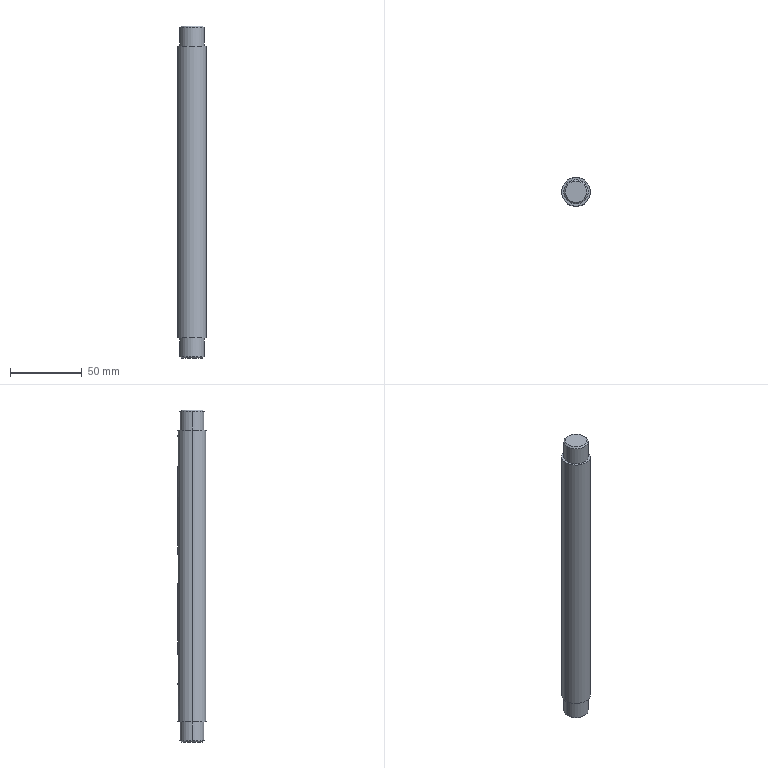Part | NX | features BREP 1 | 1 solid | 32 faces | box 20 x 20 x 231.5 mm | volume 68985 mm3 | cylinder 15 | plane 13 | cone 4 | commonest cylinder face diameters 6 x9 17 x4 20 x2
STEP:
#1=CARTESIAN_POINT('',(8.5,0.,-114.75));
#2=VERTEX_POINT('',#1);
#3=CARTESIAN_POINT('',(-8.5,0.,-114.75));
#4=VERTEX_POINT('',#3);
#5=CARTESIAN_POINT('',(0.,0.,-114.75));
#6=DIRECTION('',(0.,0.,-1.));
#7=DIRECTION('',(1.,0.,0.));
#8=AXIS2_PLACEMENT_3D('',#5,#6,#7);
#9=CIRCLE('',#8,8.5);
#10=EDGE_CURVE('',#2,#4,#9,.T.);
#11=ORIENTED_EDGE('',*,*,#10,.F.);
#12=CARTESIAN_POINT('',(8.5,0.,-101.75));
#13=VERTEX_POINT('',#12);
#14=CARTESIAN_POINT('',(8.5,0.,-101.75));
#15=DIRECTION('',(0.,0.,-1.));
#16=VECTOR('',#15,1000.);
#17=LINE('',#14,#16);
#18=EDGE_CURVE('',#13,#2,#17,.T.);
#19=ORIENTED_EDGE('',*,*,#18,.F.);
#20=CARTESIAN_POINT('',(-8.5,0.,-101.75));
#21=VERTEX_POINT('',#20);
#22=CARTESIAN_POINT('',(0.,0.,-101.75));
#23=DIRECTION('',(0.,0.,1.));
#24=DIRECTION('',(-1.,0.,0.));
#25=AXIS2_PLACEMENT_3D('',#22,#23,#24);
#26=CIRCLE('',#25,8.5);
#27=EDGE_CURVE('',#21,#13,#26,.T.);
#28=ORIENTED_EDGE('',*,*,#27,.F.);
#29=CARTESIAN_POINT('',(-8.5,0.,-101.75));
#30=DIRECTION('',(0.,0.,-1.));
#31=VECTOR('',#30,1000.);
#32=LINE('',#29,#31);
#33=EDGE_CURVE('',#21,#4,#32,.T.);
#34=ORIENTED_EDGE('',*,*,#33,.T.);
#35=EDGE_LOOP('',(#11,#19,#28,#34));
#36=FACE_BOUND('',#35,.T.);
#37=CARTESIAN_POINT('',(0.,0.,-115.75));
#38=DIRECTION('',(0.,0.,1.));
#39=DIRECTION('',(-1.,0.,0.));
#40=AXIS2_PLACEMENT_3D('',#37,#38,#39);
#41=CYLINDRICAL_SURFACE('',#40,8.5);
#42=ADVANCED_FACE('',(#36),#41,.T.);
#43=ORIENTED_EDGE('',*,*,#33,.F.);
#44=CARTESIAN_POINT('',(0.,0.,-101.75));
#45=DIRECTION('',(0.,0.,1.));
#46=DIRECTION('',(1.,0.,0.));
#47=AXIS2_PLACEMENT_3D('',#44,#45,#46);
#48=CIRCLE('',#47,8.5);
#49=EDGE_CURVE('',#13,#21,#48,.T.);
#50=ORIENTED_EDGE('',*,*,#49,.F.);
#51=ORIENTED_EDGE('',*,*,#18,.T.);
#52=CARTESIAN_POINT('',(0.,0.,-114.75));
#53=DIRECTION('',(0.,0.,-1.));
#54=DIRECTION('',(-1.,0.,0.));
#55=AXIS2_PLACEMENT_3D('',#52,#53,#54);
#56=CIRCLE('',#55,8.5);
#57=EDGE_CURVE('',#4,#2,#56,.T.);
#58=ORIENTED_EDGE('',*,*,#57,.F.);
#59=EDGE_LOOP('',(#43,#50,#51,#58));
#60=FACE_BOUND('',#59,.T.);
#61=CARTESIAN_POINT('',(0.,0.,-115.75));
#62=DIRECTION('',(0.,0.,1.));
#63=DIRECTION('',(-1.,0.,0.));
#64=AXIS2_PLACEMENT_3D('',#61,#62,#63);
#65=CYLINDRICAL_SURFACE('',#64,8.5);
#66=ADVANCED_FACE('',(#60),#65,.T.);
#67=CARTESIAN_POINT('',(-7.5,0.,-115.75));
#68=VERTEX_POINT('',#67);
#69=CARTESIAN_POINT('',(-8.5,0.,-114.75));
#70=DIRECTION('',(0.7071,0.,-0.7071));
#71=VECTOR('',#70,1000.);
#72=LINE('',#69,#71);
#73=EDGE_CURVE('',#68,#4,#72,.F.);
#74=ORIENTED_EDGE('',*,*,#73,.T.);
#75=ORIENTED_EDGE('',*,*,#57,.T.);
#76=CARTESIAN_POINT('',(7.5,0.,-115.75));
#77=VERTEX_POINT('',#76);
#78=CARTESIAN_POINT('',(8.5,0.,-114.75));
#79=DIRECTION('',(-0.7071,0.,-0.7071));
#80=VECTOR('',#79,1000.);
#81=LINE('',#78,#80);
#82=EDGE_CURVE('',#77,#2,#81,.F.);
#83=ORIENTED_EDGE('',*,*,#82,.F.);
#84=CARTESIAN_POINT('',(0.,0.,-115.75));
#85=DIRECTION('',(0.,0.,-1.));
#86=DIRECTION('',(-1.,0.,0.));
#87=AXIS2_PLACEMENT_3D('',#84,#85,#86);
#88=CIRCLE('',#87,7.5);
#89=EDGE_CURVE('',#68,#77,#88,.T.);
#90=ORIENTED_EDGE('',*,*,#89,.F.);
#91=EDGE_LOOP('',(#74,#75,#83,#90));
#92=FACE_BOUND('',#91,.T.);
#93=CARTESIAN_POINT('',(0.,0.,-115.25));
#94=DIRECTION('',(0.,0.,1.));
#95=DIRECTION('',(-1.,0.,0.));
#96=AXIS2_PLACEMENT_3D('',#93,#94,#95);
#97=CONICAL_SURFACE('',#96,8.,0.7854);
#98=ADVANCED_FACE('',(#92),#97,.T.);
#99=ORIENTED_EDGE('',*,*,#89,.T.);
#100=CARTESIAN_POINT('',(0.,0.,-115.75));
#101=DIRECTION('',(0.,0.,-1.));
#102=DIRECTION('',(1.,0.,0.));
#103=AXIS2_PLACEMENT_3D('',#100,#101,#102);
#104=CIRCLE('',#103,7.5);
#105=EDGE_CURVE('',#77,#68,#104,.T.);
#106=ORIENTED_EDGE('',*,*,#105,.T.);
#107=EDGE_LOOP('',(#99,#106));
#108=FACE_BOUND('',#107,.T.);
#109=CARTESIAN_POINT('',(0.,0.,-115.75));
#110=DIRECTION('',(0.,0.,-1.));
#111=DIRECTION('',(-1.,0.,0.));
#112=AXIS2_PLACEMENT_3D('',#109,#110,#111);
#113=PLANE('',#112);
#114=ADVANCED_FACE('',(#108),#113,.T.);
#115=ORIENTED_EDGE('',*,*,#105,.F.);
#116=ORIENTED_EDGE('',*,*,#82,.T.);
#117=ORIENTED_EDGE('',*,*,#10,.T.);
#118=ORIENTED_EDGE('',*,*,#73,.F.);
#119=EDGE_LOOP('',(#115,#116,#117,#118));
#120=FACE_BOUND('',#119,.T.);
#121=CARTESIAN_POINT('',(0.,0.,-115.25));
#122=DIRECTION('',(0.,0.,1.));
#123=DIRECTION('',(-1.,0.,0.));
#124=AXIS2_PLACEMENT_3D('',#121,#122,#123);
#125=CONICAL_SURFACE('',#124,8.,0.7854);
#126=ADVANCED_FACE('',(#120),#125,.T.);
#127=CARTESIAN_POINT('',(-10.,0.,-101.75));
#128=VERTEX_POINT('',#127);
#129=CARTESIAN_POINT('',(10.,0.,-101.75));
#130=VERTEX_POINT('',#129);
#131=CARTESIAN_POINT('',(0.,0.,-101.75));
#132=DIRECTION('',(0.,0.,-1.));
#133=DIRECTION('',(-1.,0.,0.));
#134=AXIS2_PLACEMENT_3D('',#131,#132,#133);
#135=CIRCLE('',#134,10.);
#136=EDGE_CURVE('',#128,#130,#135,.T.);
#137=ORIENTED_EDGE('',*,*,#136,.T.);
#138=CARTESIAN_POINT('',(0.,0.,-101.75));
#139=DIRECTION('',(0.,0.,-1.));
#140=DIRECTION('',(1.,0.,0.));
#141=AXIS2_PLACEMENT_3D('',#138,#139,#140);
#142=CIRCLE('',#141,10.);
#143=EDGE_CURVE('',#130,#128,#142,.T.);
#144=ORIENTED_EDGE('',*,*,#143,.T.);
#145=EDGE_LOOP('',(#137,#144));
#146=FACE_BOUND('',#145,.T.);
#147=ORIENTED_EDGE('',*,*,#27,.T.);
#148=ORIENTED_EDGE('',*,*,#49,.T.);
#149=EDGE_LOOP('',(#147,#148));
#150=FACE_BOUND('',#149,.T.);
#151=CARTESIAN_POINT('',(0.,0.,-101.75));
#152=DIRECTION('',(0.,0.,1.));
#153=DIRECTION('',(-1.,0.,0.));
#154=AXIS2_PLACEMENT_3D('',#151,#152,#153);
#155=PLANE('',#154);
#156=ADVANCED_FACE('',(#146,#150),#155,.F.);
#157=CARTESIAN_POINT('',(-10.,0.,101.75));
#158=VERTEX_POINT('',#157);
#159=CARTESIAN_POINT('',(10.,0.,101.75));
#160=VERTEX_POINT('',#159);
#161=CARTESIAN_POINT('',(0.,0.,101.75));
#162=DIRECTION('',(0.,0.,1.));
#163=DIRECTION('',(-1.,0.,0.));
#164=AXIS2_PLACEMENT_3D('',#161,#162,#163);
#165=CIRCLE('',#164,10.);
#166=EDGE_CURVE('',#158,#160,#165,.T.);
#167=ORIENTED_EDGE('',*,*,#166,.F.);
#168=CARTESIAN_POINT('',(-10.,0.,-101.75));
#169=DIRECTION('',(0.,0.,1.));
#170=VECTOR('',#169,1000.);
#171=LINE('',#168,#170);
#172=EDGE_CURVE('',#158,#128,#171,.F.);
#173=ORIENTED_EDGE('',*,*,#172,.T.);
#174=ORIENTED_EDGE('',*,*,#143,.F.);
#175=CARTESIAN_POINT('',(10.,0.,-101.75));
#176=DIRECTION('',(0.,0.,1.));
#177=VECTOR('',#176,1000.);
#178=LINE('',#175,#177);
#179=EDGE_CURVE('',#160,#130,#178,.F.);
#180=ORIENTED_EDGE('',*,*,#179,.F.);
#181=EDGE_LOOP('',(#167,#173,#174,#180));
#182=FACE_BOUND('',#181,.T.);
#183=CARTESIAN_POINT('',(0.,0.,101.75));
#184=DIRECTION('',(0.,0.,-1.));
#185=DIRECTION('',(1.,0.,0.));
#186=AXIS2_PLACEMENT_3D('',#183,#184,#185);
#187=CYLINDRICAL_SURFACE('',#186,10.);
#188=ADVANCED_FACE('',(#182),#187,.T.);
#189=ORIENTED_EDGE('',*,*,#179,.T.);
#190=ORIENTED_EDGE('',*,*,#136,.F.);
#191=ORIENTED_EDGE('',*,*,#172,.F.);
#192=CARTESIAN_POINT('',(0.,0.,101.75));
#193=DIRECTION('',(0.,0.,1.));
#194=DIRECTION('',(1.,0.,0.));
#195=AXIS2_PLACEMENT_3D('',#192,#193,#194);
#196=CIRCLE('',#195,10.);
#197=EDGE_CURVE('',#160,#158,#196,.T.);
#198=ORIENTED_EDGE('',*,*,#197,.F.);
#199=EDGE_LOOP('',(#189,#190,#191,#198));
#200=FACE_BOUND('',#199,.T.);
#201=CARTESIAN_POINT('',(-3.,9.539,94.75));
#202=VERTEX_POINT('',#201);
#203=CARTESIAN_POINT('',(0.,10.,97.75));
#204=VERTEX_POINT('',#203);
#205=CARTESIAN_POINT('',(-3.,9.539,94.75));
#206=CARTESIAN_POINT('',(-3.,9.539,95.547));
#207=CARTESIAN_POINT('',(-2.345,9.775,97.093));
#208=CARTESIAN_POINT('',(-0.7973,10.,97.75));
#209=CARTESIAN_POINT('',(0.,10.,97.75));
#210=B_SPLINE_CURVE_WITH_KNOTS('',3,(#205,#206,#207,#208,#209),.UNSPECIFIED.,.F.,.F.,(4,1,4),(0.,0.002357,0.004714),.UNSPECIFIED.);
#211=EDGE_CURVE('',#202,#204,#210,.T.);
#212=ORIENTED_EDGE('',*,*,#211,.F.);
#213=CARTESIAN_POINT('',(-3.,9.539,78.75));
#214=VERTEX_POINT('',#213);
#215=CARTESIAN_POINT('',(-3.,9.539,94.75));
#216=DIRECTION('',(0.,0.,-1.));
#217=VECTOR('',#216,1000.);
#218=LINE('',#215,#217);
#219=EDGE_CURVE('',#202,#214,#218,.T.);
#220=ORIENTED_EDGE('',*,*,#219,.T.);
#221=CARTESIAN_POINT('',(3.,9.539,78.75));
#222=VERTEX_POINT('',#221);
#223=CARTESIAN_POINT('',(3.,9.539,78.75));
#224=CARTESIAN_POINT('',(3.,9.539,77.952));
#225=CARTESIAN_POINT('',(2.35,9.775,76.406));
#226=CARTESIAN_POINT('',(0.004774,10.112,75.422));
#227=CARTESIAN_POINT('',(-2.351,9.775,76.405));
#228=CARTESIAN_POINT('',(-3.,9.539,77.952));
#229=CARTESIAN_POINT('',(-3.,9.539,78.75));
#230=B_SPLINE_CURVE_WITH_KNOTS('',3,(#223,#224,#225,#226,#227,#228,#229),.UNSPECIFIED.,.F.,.F.,(4,1,1,1,4),(0.,0.002358,0.004715,0.007073,0.009431),.UNSPECIFIED.);
#231=EDGE_CURVE('',#222,#214,#230,.T.);
#232=ORIENTED_EDGE('',*,*,#231,.F.);
#233=CARTESIAN_POINT('',(3.,9.539,94.75));
#234=VERTEX_POINT('',#233);
#235=CARTESIAN_POINT('',(3.,9.539,78.75));
#236=DIRECTION('',(0.,0.,1.));
#237=VECTOR('',#236,1000.);
#238=LINE('',#235,#237);
#239=EDGE_CURVE('',#222,#234,#238,.T.);
#240=ORIENTED_EDGE('',*,*,#239,.T.);
#241=CARTESIAN_POINT('',(0.,10.,97.75));
#242=CARTESIAN_POINT('',(0.7973,10.,97.75));
#243=CARTESIAN_POINT('',(2.343,9.775,97.095));
#244=CARTESIAN_POINT('',(3.,9.539,95.547));
#245=CARTESIAN_POINT('',(3.,9.539,94.75));
#246=B_SPLINE_CURVE_WITH_KNOTS('',3,(#241,#242,#243,#244,#245),.UNSPECIFIED.,.F.,.F.,(4,1,4),(0.,0.002357,0.004714),.UNSPECIFIED.);
#247=EDGE_CURVE('',#204,#234,#246,.T.);
#248=ORIENTED_EDGE('',*,*,#247,.F.);
#249=EDGE_LOOP('',(#212,#220,#232,#240,#248));
#250=FACE_BOUND('',#249,.T.);
#251=CARTESIAN_POINT('',(-3.,9.539,-56.75));
#252=VERTEX_POINT('',#251);
#253=CARTESIAN_POINT('',(0.,10.,-53.75));
#254=VERTEX_POINT('',#253);
#255=CARTESIAN_POINT('',(-3.,9.539,-56.75));
#256=CARTESIAN_POINT('',(-3.,9.539,-55.953));
#257=CARTESIAN_POINT('',(-2.345,9.775,-54.407));
#258=CARTESIAN_POINT('',(-0.7973,10.,-53.75));
#259=CARTESIAN_POINT('',(0.,10.,-53.75));
#260=B_SPLINE_CURVE_WITH_KNOTS('',3,(#255,#256,#257,#258,#259),.UNSPECIFIED.,.F.,.F.,(4,1,4),(0.,0.002357,0.004714),.UNSPECIFIED.);
#261=EDGE_CURVE('',#252,#254,#260,.T.);
#262=ORIENTED_EDGE('',*,*,#261,.F.);
#263=CARTESIAN_POINT('',(-3.,9.539,-72.75));
#264=VERTEX_POINT('',#263);
#265=CARTESIAN_POINT('',(-3.,9.539,-56.75));
#266=DIRECTION('',(0.,0.,-1.));
#267=VECTOR('',#266,1000.);
#268=LINE('',#265,#267);
#269=EDGE_CURVE('',#252,#264,#268,.T.);
#270=ORIENTED_EDGE('',*,*,#269,.T.);
#271=CARTESIAN_POINT('',(3.,9.539,-72.75));
#272=VERTEX_POINT('',#271);
#273=CARTESIAN_POINT('',(3.,9.539,-72.75));
#274=CARTESIAN_POINT('',(3.,9.539,-73.548));
#275=CARTESIAN_POINT('',(2.35,9.775,-75.094));
#276=CARTESIAN_POINT('',(0.004774,10.112,-76.078));
#277=CARTESIAN_POINT('',(-2.351,9.775,-75.095));
#278=CARTESIAN_POINT('',(-3.,9.539,-73.548));
#279=CARTESIAN_POINT('',(-3.,9.539,-72.75));
#280=B_SPLINE_CURVE_WITH_KNOTS('',3,(#273,#274,#275,#276,#277,#278,#279),.UNSPECIFIED.,.F.,.F.,(4,1,1,1,4),(0.,0.002358,0.004715,0.007073,0.009431),.UNSPECIFIED.);
#281=EDGE_CURVE('',#272,#264,#280,.T.);
#282=ORIENTED_EDGE('',*,*,#281,.F.);
#283=CARTESIAN_POINT('',(3.,9.539,-56.75));
#284=VERTEX_POINT('',#283);
#285=CARTESIAN_POINT('',(3.,9.539,-72.75));
#286=DIRECTION('',(0.,0.,1.));
#287=VECTOR('',#286,1000.);
#288=LINE('',#285,#287);
#289=EDGE_CURVE('',#272,#284,#288,.T.);
#290=ORIENTED_EDGE('',*,*,#289,.T.);
#291=CARTESIAN_POINT('',(0.,10.,-53.75));
#292=CARTESIAN_POINT('',(0.7973,10.,-53.75));
#293=CARTESIAN_POINT('',(2.343,9.775,-54.405));
#294=CARTESIAN_POINT('',(3.,9.539,-55.953));
#295=CARTESIAN_POINT('',(3.,9.539,-56.75));
#296=B_SPLINE_CURVE_WITH_KNOTS('',3,(#291,#292,#293,#294,#295),.UNSPECIFIED.,.F.,.F.,(4,1,4),(0.,0.002357,0.004714),.UNSPECIFIED.);
#297=EDGE_CURVE('',#254,#284,#296,.T.);
#298=ORIENTED_EDGE('',*,*,#297,.F.);
#299=EDGE_LOOP('',(#262,#270,#282,#290,#298));
#300=FACE_BOUND('',#299,.T.);
#301=CARTESIAN_POINT('',(-3.,9.539,13.));
#302=VERTEX_POINT('',#301);
#303=CARTESIAN_POINT('',(0.,10.,16.));
#304=VERTEX_POINT('',#303);
#305=CARTESIAN_POINT('',(-3.,9.539,13.));
#306=CARTESIAN_POINT('',(-3.,9.539,13.797));
#307=CARTESIAN_POINT('',(-2.345,9.775,15.343));
#308=CARTESIAN_POINT('',(-0.7973,10.,16.));
#309=CARTESIAN_POINT('',(0.,10.,16.));
#310=B_SPLINE_CURVE_WITH_KNOTS('',3,(#305,#306,#307,#308,#309),.UNSPECIFIED.,.F.,.F.,(4,1,4),(0.,0.002357,0.004714),.UNSPECIFIED.);
#311=EDGE_CURVE('',#302,#304,#310,.T.);
#312=ORIENTED_EDGE('',*,*,#311,.F.);
#313=CARTESIAN_POINT('',(-3.,9.539,-3.));
#314=VERTEX_POINT('',#313);
#315=CARTESIAN_POINT('',(-3.,9.539,13.));
#316=DIRECTION('',(0.,0.,-1.));
#317=VECTOR('',#316,1000.);
#318=LINE('',#315,#317);
#319=EDGE_CURVE('',#302,#314,#318,.T.);
#320=ORIENTED_EDGE('',*,*,#319,.T.);
#321=CARTESIAN_POINT('',(3.,9.539,-3.));
#322=VERTEX_POINT('',#321);
#323=CARTESIAN_POINT('',(3.,9.539,-3.));
#324=CARTESIAN_POINT('',(3.,9.539,-3.798));
#325=CARTESIAN_POINT('',(2.35,9.775,-5.344));
#326=CARTESIAN_POINT('',(0.004774,10.112,-6.328));
#327=CARTESIAN_POINT('',(-2.351,9.775,-5.345));
#328=CARTESIAN_POINT('',(-3.,9.539,-3.798));
#329=CARTESIAN_POINT('',(-3.,9.539,-3.));
#330=B_SPLINE_CURVE_WITH_KNOTS('',3,(#323,#324,#325,#326,#327,#328,#329),.UNSPECIFIED.,.F.,.F.,(4,1,1,1,4),(0.,0.002358,0.004715,0.007073,0.009431),.UNSPECIFIED.);
#331=EDGE_CURVE('',#322,#314,#330,.T.);
#332=ORIENTED_EDGE('',*,*,#331,.F.);
#333=CARTESIAN_POINT('',(3.,9.539,13.));
#334=VERTEX_POINT('',#333);
#335=CARTESIAN_POINT('',(3.,9.539,-3.));
#336=DIRECTION('',(0.,0.,1.));
#337=VECTOR('',#336,1000.);
#338=LINE('',#335,#337);
#339=EDGE_CURVE('',#322,#334,#338,.T.);
#340=ORIENTED_EDGE('',*,*,#339,.T.);
#341=CARTESIAN_POINT('',(0.,10.,16.));
#342=CARTESIAN_POINT('',(0.7973,10.,16.));
#343=CARTESIAN_POINT('',(2.343,9.775,15.345));
#344=CARTESIAN_POINT('',(3.,9.539,13.797));
#345=CARTESIAN_POINT('',(3.,9.539,13.));
#346=B_SPLINE_CURVE_WITH_KNOTS('',3,(#341,#342,#343,#344,#345),.UNSPECIFIED.,.F.,.F.,(4,1,4),(0.,0.002357,0.004714),.UNSPECIFIED.);
#347=EDGE_CURVE('',#304,#334,#346,.T.);
#348=ORIENTED_EDGE('',*,*,#347,.F.);
#349=EDGE_LOOP('',(#312,#320,#332,#340,#348));
#350=FACE_BOUND('',#349,.T.);
#351=CARTESIAN_POINT('',(0.,0.,101.75));
#352=DIRECTION('',(0.,0.,-1.));
#353=DIRECTION('',(1.,0.,0.));
#354=AXIS2_PLACEMENT_3D('',#351,#352,#353);
#355=CYLINDRICAL_SURFACE('',#354,10.);
#356=ADVANCED_FACE('',(#200,#250,#300,#350),#355,.T.);
#357=ORIENTED_EDGE('',*,*,#197,.T.);
#358=ORIENTED_EDGE('',*,*,#166,.T.);
#359=EDGE_LOOP('',(#357,#358));
#360=FACE_BOUND('',#359,.T.);
#361=CARTESIAN_POINT('',(-8.5,0.,101.75));
#362=VERTEX_POINT('',#361);
#363=CARTESIAN_POINT('',(8.5,0.,101.75));
#364=VERTEX_POINT('',#363);
#365=CARTESIAN_POINT('',(0.,0.,101.75));
#366=DIRECTION('',(0.,0.,-1.));
#367=DIRECTION('',(-1.,0.,0.));
#368=AXIS2_PLACEMENT_3D('',#365,#366,#367);
#369=CIRCLE('',#368,8.5);
#370=EDGE_CURVE('',#362,#364,#369,.T.);
#371=ORIENTED_EDGE('',*,*,#370,.T.);
#372=CARTESIAN_POINT('',(0.,0.,101.75));
#373=DIRECTION('',(0.,0.,-1.));
#374=DIRECTION('',(1.,0.,0.));
#375=AXIS2_PLACEMENT_3D('',#372,#373,#374);
#376=CIRCLE('',#375,8.5);
#377=EDGE_CURVE('',#364,#362,#376,.T.);
#378=ORIENTED_EDGE('',*,*,#377,.T.);
#379=EDGE_LOOP('',(#371,#378));
#380=FACE_BOUND('',#379,.T.);
#381=CARTESIAN_POINT('',(0.,0.,101.75));
#382=DIRECTION('',(0.,0.,1.));
#383=DIRECTION('',(-1.,0.,0.));
#384=AXIS2_PLACEMENT_3D('',#381,#382,#383);
#385=PLANE('',#384);
#386=ADVANCED_FACE('',(#360,#380),#385,.T.);
#387=CARTESIAN_POINT('',(-8.5,0.,114.75));
#388=VERTEX_POINT('',#387);
#389=CARTESIAN_POINT('',(8.5,0.,114.75));
#390=VERTEX_POINT('',#389);
#391=CARTESIAN_POINT('',(0.,0.,114.75));
#392=DIRECTION('',(0.,0.,1.));
#393=DIRECTION('',(-1.,0.,0.));
#394=AXIS2_PLACEMENT_3D('',#391,#392,#393);
#395=CIRCLE('',#394,8.5);
#396=EDGE_CURVE('',#388,#390,#395,.T.);
#397=ORIENTED_EDGE('',*,*,#396,.F.);
#398=CARTESIAN_POINT('',(-8.5,0.,101.75));
#399=DIRECTION('',(0.,0.,1.));
#400=VECTOR('',#399,1000.);
#401=LINE('',#398,#400);
#402=EDGE_CURVE('',#388,#362,#401,.F.);
#403=ORIENTED_EDGE('',*,*,#402,.T.);
#404=ORIENTED_EDGE('',*,*,#377,.F.);
#405=CARTESIAN_POINT('',(8.5,0.,101.75));
#406=DIRECTION('',(0.,0.,1.));
#407=VECTOR('',#406,1000.);
#408=LINE('',#405,#407);
#409=EDGE_CURVE('',#390,#364,#408,.F.);
#410=ORIENTED_EDGE('',*,*,#409,.F.);
#411=EDGE_LOOP('',(#397,#403,#404,#410));
#412=FACE_BOUND('',#411,.T.);
#413=CARTESIAN_POINT('',(0.,0.,115.75));
#414=DIRECTION('',(0.,0.,-1.));
#415=DIRECTION('',(1.,0.,0.));
#416=AXIS2_PLACEMENT_3D('',#413,#414,#415);
#417=CYLINDRICAL_SURFACE('',#416,8.5);
#418=ADVANCED_FACE('',(#412),#417,.T.);
#419=ORIENTED_EDGE('',*,*,#409,.T.);
#420=ORIENTED_EDGE('',*,*,#370,.F.);
#421=ORIENTED_EDGE('',*,*,#402,.F.);
#422=CARTESIAN_POINT('',(0.,0.,114.75));
#423=DIRECTION('',(0.,0.,1.));
#424=DIRECTION('',(1.,0.,0.));
#425=AXIS2_PLACEMENT_3D('',#422,#423,#424);
#426=CIRCLE('',#425,8.5);
#427=EDGE_CURVE('',#390,#388,#426,.T.);
#428=ORIENTED_EDGE('',*,*,#427,.F.);
#429=EDGE_LOOP('',(#419,#420,#421,#428));
#430=FACE_BOUND('',#429,.T.);
#431=CARTESIAN_POINT('',(0.,0.,115.75));
#432=DIRECTION('',(0.,0.,-1.));
#433=DIRECTION('',(1.,0.,0.));
#434=AXIS2_PLACEMENT_3D('',#431,#432,#433);
#435=CYLINDRICAL_SURFACE('',#434,8.5);
#436=ADVANCED_FACE('',(#430),#435,.T.);
#437=CARTESIAN_POINT('',(7.5,0.,115.75));
#438=VERTEX_POINT('',#437);
#439=CARTESIAN_POINT('',(8.5,0.,114.75));
#440=DIRECTION('',(-0.7071,0.,0.7071));
#441=VECTOR('',#440,1000.);
#442=LINE('',#439,#441);
#443=EDGE_CURVE('',#390,#438,#442,.T.);
#444=ORIENTED_EDGE('',*,*,#443,.F.);
#445=ORIENTED_EDGE('',*,*,#427,.T.);
#446=CARTESIAN_POINT('',(-7.5,0.,115.75));
#447=VERTEX_POINT('',#446);
#448=CARTESIAN_POINT('',(-8.5,0.,114.75));
#449=DIRECTION('',(0.7071,0.,0.7071));
#450=VECTOR('',#449,1000.);
#451=LINE('',#448,#450);
#452=EDGE_CURVE('',#388,#447,#451,.T.);
#453=ORIENTED_EDGE('',*,*,#452,.T.);
#454=CARTESIAN_POINT('',(0.,0.,115.75));
#455=DIRECTION('',(0.,0.,1.));
#456=DIRECTION('',(1.,0.,0.));
#457=AXIS2_PLACEMENT_3D('',#454,#455,#456);
#458=CIRCLE('',#457,7.5);
#459=EDGE_CURVE('',#438,#447,#458,.T.);
#460=ORIENTED_EDGE('',*,*,#459,.F.);
#461=EDGE_LOOP('',(#444,#445,#453,#460));
#462=FACE_BOUND('',#461,.T.);
#463=CARTESIAN_POINT('',(0.,0.,115.25));
#464=DIRECTION('',(0.,0.,-1.));
#465=DIRECTION('',(1.,0.,0.));
#466=AXIS2_PLACEMENT_3D('',#463,#464,#465);
#467=CONICAL_SURFACE('',#466,8.,0.7854);
#468=ADVANCED_FACE('',(#462),#467,.T.);
#469=ORIENTED_EDGE('',*,*,#459,.T.);
#470=CARTESIAN_POINT('',(0.,0.,115.75));
#471=DIRECTION('',(0.,0.,1.));
#472=DIRECTION('',(-1.,0.,0.));
#473=AXIS2_PLACEMENT_3D('',#470,#471,#472);
#474=CIRCLE('',#473,7.5);
#475=EDGE_CURVE('',#447,#438,#474,.T.);
#476=ORIENTED_EDGE('',*,*,#475,.T.);
#477=EDGE_LOOP('',(#469,#476));
#478=FACE_BOUND('',#477,.T.);
#479=CARTESIAN_POINT('',(0.,0.,115.75));
#480=DIRECTION('',(0.,0.,1.));
#481=DIRECTION('',(-1.,0.,0.));
#482=AXIS2_PLACEMENT_3D('',#479,#480,#481);
#483=PLANE('',#482);
#484=ADVANCED_FACE('',(#478),#483,.T.);
#485=ORIENTED_EDGE('',*,*,#475,.F.);
#486=ORIENTED_EDGE('',*,*,#452,.F.);
#487=ORIENTED_EDGE('',*,*,#396,.T.);
#488=ORIENTED_EDGE('',*,*,#443,.T.);
#489=EDGE_LOOP('',(#485,#486,#487,#488));
#490=FACE_BOUND('',#489,.T.);
#491=CARTESIAN_POINT('',(0.,0.,115.25));
#492=DIRECTION('',(0.,0.,-1.));
#493=DIRECTION('',(1.,0.,0.));
#494=AXIS2_PLACEMENT_3D('',#491,#492,#493);
#495=CONICAL_SURFACE('',#494,8.,0.7854);
#496=ADVANCED_FACE('',(#490),#495,.T.);
#497=CARTESIAN_POINT('',(0.,6.5,97.75));
#498=VERTEX_POINT('',#497);
#499=CARTESIAN_POINT('',(0.,10.,97.75));
#500=DIRECTION('',(0.,-1.,0.));
#501=VECTOR('',#500,1000.);
#502=LINE('',#499,#501);
#503=EDGE_CURVE('',#204,#498,#502,.T.);
#504=ORIENTED_EDGE('',*,*,#503,.F.);
#505=ORIENTED_EDGE('',*,*,#247,.T.);
#506=CARTESIAN_POINT('',(3.,6.5,94.75));
#507=VERTEX_POINT('',#506);
#508=CARTESIAN_POINT('',(3.,9.539,94.75));
#509=DIRECTION('',(0.,-1.,0.));
#510=VECTOR('',#509,1000.);
#511=LINE('',#508,#510);
#512=EDGE_CURVE('',#234,#507,#511,.T.);
#513=ORIENTED_EDGE('',*,*,#512,.T.);
#514=CARTESIAN_POINT('',(0.,6.5,94.75));
#515=DIRECTION('',(0.,1.,0.));
#516=DIRECTION('',(0.,0.,1.));
#517=AXIS2_PLACEMENT_3D('',#514,#515,#516);
#518=CIRCLE('',#517,3.);
#519=EDGE_CURVE('',#498,#507,#518,.T.);
#520=ORIENTED_EDGE('',*,*,#519,.F.);
#521=EDGE_LOOP('',(#504,#505,#513,#520));
#522=FACE_BOUND('',#521,.T.);
#523=CARTESIAN_POINT('',(0.,6.5,94.75));
#524=DIRECTION('',(0.,1.,0.));
#525=DIRECTION('',(0.,0.,-1.));
#526=AXIS2_PLACEMENT_3D('',#523,#524,#525);
#527=CYLINDRICAL_SURFACE('',#526,3.);
#528=ADVANCED_FACE('',(#522),#527,.F.);
#529=CARTESIAN_POINT('',(0.,6.5,75.75));
#530=VERTEX_POINT('',#529);
#531=CARTESIAN_POINT('',(-3.,6.5,78.75));
#532=VERTEX_POINT('',#531);
#533=CARTESIAN_POINT('',(0.,6.5,78.75));
#534=DIRECTION('',(0.,1.,0.));
#535=DIRECTION('',(0.,0.,-1.));
#536=AXIS2_PLACEMENT_3D('',#533,#534,#535);
#537=CIRCLE('',#536,3.);
#538=EDGE_CURVE('',#530,#532,#537,.T.);
#539=ORIENTED_EDGE('',*,*,#538,.T.);
#540=CARTESIAN_POINT('',(-3.,6.5,94.75));
#541=VERTEX_POINT('',#540);
#542=CARTESIAN_POINT('',(-3.,6.5,94.75));
#543=DIRECTION('',(0.,0.,-1.));
#544=VECTOR('',#543,1000.);
#545=LINE('',#542,#544);
#546=EDGE_CURVE('',#541,#532,#545,.T.);
#547=ORIENTED_EDGE('',*,*,#546,.F.);
#548=CARTESIAN_POINT('',(0.,6.5,94.75));
#549=DIRECTION('',(0.,1.,0.));
#550=DIRECTION('',(-1.,0.,0.));
#551=AXIS2_PLACEMENT_3D('',#548,#549,#550);
#552=CIRCLE('',#551,3.);
#553=EDGE_CURVE('',#541,#498,#552,.T.);
#554=ORIENTED_EDGE('',*,*,#553,.T.);
#555=ORIENTED_EDGE('',*,*,#519,.T.);
#556=CARTESIAN_POINT('',(3.,6.5,78.75));
#557=VERTEX_POINT('',#556);
#558=CARTESIAN_POINT('',(3.,6.5,78.75));
#559=DIRECTION('',(0.,0.,1.));
#560=VECTOR('',#559,1000.);
#561=LINE('',#558,#560);
#562=EDGE_CURVE('',#557,#507,#561,.T.);
#563=ORIENTED_EDGE('',*,*,#562,.F.);
#564=CARTESIAN_POINT('',(0.,6.5,78.75));
#565=DIRECTION('',(0.,1.,0.));
#566=DIRECTION('',(1.,0.,0.));
#567=AXIS2_PLACEMENT_3D('',#564,#565,#566);
#568=CIRCLE('',#567,3.);
#569=EDGE_CURVE('',#557,#530,#568,.T.);
#570=ORIENTED_EDGE('',*,*,#569,.T.);
#571=EDGE_LOOP('',(#539,#547,#554,#555,#563,#570));
#572=FACE_BOUND('',#571,.T.);
#573=CARTESIAN_POINT('',(0.,6.5,78.75));
#574=DIRECTION('',(0.,1.,0.));
#575=DIRECTION('',(0.,0.,-1.));
#576=AXIS2_PLACEMENT_3D('',#573,#574,#575);
#577=PLANE('',#576);
#578=ADVANCED_FACE('',(#572),#577,.T.);
#579=ORIENTED_EDGE('',*,*,#538,.F.);
#580=ORIENTED_EDGE('',*,*,#569,.F.);
#581=CARTESIAN_POINT('',(3.,6.5,78.75));
#582=DIRECTION('',(0.,1.,0.));
#583=VECTOR('',#582,1000.);
#584=LINE('',#581,#583);
#585=EDGE_CURVE('',#557,#222,#584,.T.);
#586=ORIENTED_EDGE('',*,*,#585,.T.);
#587=ORIENTED_EDGE('',*,*,#231,.T.);
#588=CARTESIAN_POINT('',(-3.,9.539,78.75));
#589=DIRECTION('',(0.,-1.,0.));
#590=VECTOR('',#589,1000.);
#591=LINE('',#588,#590);
#592=EDGE_CURVE('',#214,#532,#591,.T.);
#593=ORIENTED_EDGE('',*,*,#592,.T.);
#594=EDGE_LOOP('',(#579,#580,#586,#587,#593));
#595=FACE_BOUND('',#594,.T.);
#596=CARTESIAN_POINT('',(0.,6.5,78.75));
#597=DIRECTION('',(0.,1.,0.));
#598=DIRECTION('',(0.,0.,-1.));
#599=AXIS2_PLACEMENT_3D('',#596,#597,#598);
#600=CYLINDRICAL_SURFACE('',#599,3.);
#601=ADVANCED_FACE('',(#595),#600,.F.);
#602=ORIENTED_EDGE('',*,*,#546,.T.);
#603=ORIENTED_EDGE('',*,*,#592,.F.);
#604=ORIENTED_EDGE('',*,*,#219,.F.);
#605=CARTESIAN_POINT('',(-3.,6.5,94.75));
#606=DIRECTION('',(0.,1.,0.));
#607=VECTOR('',#606,1000.);
#608=LINE('',#605,#607);
#609=EDGE_CURVE('',#541,#202,#608,.T.);
#610=ORIENTED_EDGE('',*,*,#609,.F.);
#611=EDGE_LOOP('',(#602,#603,#604,#610));
#612=FACE_BOUND('',#611,.T.);
#613=CARTESIAN_POINT('',(-3.,6.5,78.75));
#614=DIRECTION('',(-1.,0.,0.));
#615=DIRECTION('',(0.,0.,-1.));
#616=AXIS2_PLACEMENT_3D('',#613,#614,#615);
#617=PLANE('',#616);
#618=ADVANCED_FACE('',(#612),#617,.F.);
#619=ORIENTED_EDGE('',*,*,#553,.F.);
#620=ORIENTED_EDGE('',*,*,#609,.T.);
#621=ORIENTED_EDGE('',*,*,#211,.T.);
#622=ORIENTED_EDGE('',*,*,#503,.T.);
#623=EDGE_LOOP('',(#619,#620,#621,#622));
#624=FACE_BOUND('',#623,.T.);
#625=CARTESIAN_POINT('',(0.,6.5,94.75));
#626=DIRECTION('',(0.,1.,0.));
#627=DIRECTION('',(0.,0.,-1.));
#628=AXIS2_PLACEMENT_3D('',#625,#626,#627);
#629=CYLINDRICAL_SURFACE('',#628,3.);
#630=ADVANCED_FACE('',(#624),#629,.F.);
#631=ORIENTED_EDGE('',*,*,#562,.T.);
#632=ORIENTED_EDGE('',*,*,#512,.F.);
#633=ORIENTED_EDGE('',*,*,#239,.F.);
#634=ORIENTED_EDGE('',*,*,#585,.F.);
#635=EDGE_LOOP('',(#631,#632,#633,#634));
#636=FACE_BOUND('',#635,.T.);
#637=CARTESIAN_POINT('',(3.,6.5,78.75));
#638=DIRECTION('',(1.,0.,0.));
#639=DIRECTION('',(0.,0.,1.));
#640=AXIS2_PLACEMENT_3D('',#637,#638,#639);
#641=PLANE('',#640);
#642=ADVANCED_FACE('',(#636),#641,.F.);
#643=CARTESIAN_POINT('',(0.,6.5,-53.75));
#644=VERTEX_POINT('',#643);
#645=CARTESIAN_POINT('',(0.,10.,-53.75));
#646=DIRECTION('',(0.,-1.,0.));
#647=VECTOR('',#646,1000.);
#648=LINE('',#645,#647);
#649=EDGE_CURVE('',#254,#644,#648,.T.);
#650=ORIENTED_EDGE('',*,*,#649,.F.);
#651=ORIENTED_EDGE('',*,*,#297,.T.);
#652=CARTESIAN_POINT('',(3.,6.5,-56.75));
#653=VERTEX_POINT('',#652);
#654=CARTESIAN_POINT('',(3.,9.539,-56.75));
#655=DIRECTION('',(0.,-1.,0.));
#656=VECTOR('',#655,1000.);
#657=LINE('',#654,#656);
#658=EDGE_CURVE('',#284,#653,#657,.T.);
#659=ORIENTED_EDGE('',*,*,#658,.T.);
#660=CARTESIAN_POINT('',(0.,6.5,-56.75));
#661=DIRECTION('',(0.,1.,0.));
#662=DIRECTION('',(0.,0.,1.));
#663=AXIS2_PLACEMENT_3D('',#660,#661,#662);
#664=CIRCLE('',#663,3.);
#665=EDGE_CURVE('',#644,#653,#664,.T.);
#666=ORIENTED_EDGE('',*,*,#665,.F.);
#667=EDGE_LOOP('',(#650,#651,#659,#666));
#668=FACE_BOUND('',#667,.T.);
#669=CARTESIAN_POINT('',(0.,6.5,-56.75));
#670=DIRECTION('',(0.,1.,0.));
#671=DIRECTION('',(0.,0.,-1.));
#672=AXIS2_PLACEMENT_3D('',#669,#670,#671);
#673=CYLINDRICAL_SURFACE('',#672,3.);
#674=ADVANCED_FACE('',(#668),#673,.F.);
#675=CARTESIAN_POINT('',(0.,6.5,-75.75));
#676=VERTEX_POINT('',#675);
#677=CARTESIAN_POINT('',(-3.,6.5,-72.75));
#678=VERTEX_POINT('',#677);
#679=CARTESIAN_POINT('',(0.,6.5,-72.75));
#680=DIRECTION('',(0.,1.,0.));
#681=DIRECTION('',(0.,0.,-1.));
#682=AXIS2_PLACEMENT_3D('',#679,#680,#681);
#683=CIRCLE('',#682,3.);
#684=EDGE_CURVE('',#676,#678,#683,.T.);
#685=ORIENTED_EDGE('',*,*,#684,.T.);
#686=CARTESIAN_POINT('',(-3.,6.5,-56.75));
#687=VERTEX_POINT('',#686);
#688=CARTESIAN_POINT('',(-3.,6.5,-56.75));
#689=DIRECTION('',(0.,0.,-1.));
#690=VECTOR('',#689,1000.);
#691=LINE('',#688,#690);
#692=EDGE_CURVE('',#687,#678,#691,.T.);
#693=ORIENTED_EDGE('',*,*,#692,.F.);
#694=CARTESIAN_POINT('',(0.,6.5,-56.75));
#695=DIRECTION('',(0.,1.,0.));
#696=DIRECTION('',(-1.,0.,0.));
#697=AXIS2_PLACEMENT_3D('',#694,#695,#696);
#698=CIRCLE('',#697,3.);
#699=EDGE_CURVE('',#687,#644,#698,.T.);
#700=ORIENTED_EDGE('',*,*,#699,.T.);
#701=ORIENTED_EDGE('',*,*,#665,.T.);
#702=CARTESIAN_POINT('',(3.,6.5,-72.75));
#703=VERTEX_POINT('',#702);
#704=CARTESIAN_POINT('',(3.,6.5,-72.75));
#705=DIRECTION('',(0.,0.,1.));
#706=VECTOR('',#705,1000.);
#707=LINE('',#704,#706);
#708=EDGE_CURVE('',#703,#653,#707,.T.);
#709=ORIENTED_EDGE('',*,*,#708,.F.);
#710=CARTESIAN_POINT('',(0.,6.5,-72.75));
#711=DIRECTION('',(0.,1.,0.));
#712=DIRECTION('',(1.,0.,0.));
#713=AXIS2_PLACEMENT_3D('',#710,#711,#712);
#714=CIRCLE('',#713,3.);
#715=EDGE_CURVE('',#703,#676,#714,.T.);
#716=ORIENTED_EDGE('',*,*,#715,.T.);
#717=EDGE_LOOP('',(#685,#693,#700,#701,#709,#716));
#718=FACE_BOUND('',#717,.T.);
#719=CARTESIAN_POINT('',(0.,6.5,-72.75));
#720=DIRECTION('',(0.,1.,0.));
#721=DIRECTION('',(0.,0.,-1.));
#722=AXIS2_PLACEMENT_3D('',#719,#720,#721);
#723=PLANE('',#722);
#724=ADVANCED_FACE('',(#718),#723,.T.);
#725=ORIENTED_EDGE('',*,*,#684,.F.);
#726=ORIENTED_EDGE('',*,*,#715,.F.);
#727=CARTESIAN_POINT('',(3.,6.5,-72.75));
#728=DIRECTION('',(0.,1.,0.));
#729=VECTOR('',#728,1000.);
#730=LINE('',#727,#729);
#731=EDGE_CURVE('',#703,#272,#730,.T.);
#732=ORIENTED_EDGE('',*,*,#731,.T.);
#733=ORIENTED_EDGE('',*,*,#281,.T.);
#734=CARTESIAN_POINT('',(-3.,9.539,-72.75));
#735=DIRECTION('',(0.,-1.,0.));
#736=VECTOR('',#735,1000.);
#737=LINE('',#734,#736);
#738=EDGE_CURVE('',#264,#678,#737,.T.);
#739=ORIENTED_EDGE('',*,*,#738,.T.);
#740=EDGE_LOOP('',(#725,#726,#732,#733,#739));
#741=FACE_BOUND('',#740,.T.);
#742=CARTESIAN_POINT('',(0.,6.5,-72.75));
#743=DIRECTION('',(0.,1.,0.));
#744=DIRECTION('',(0.,0.,-1.));
#745=AXIS2_PLACEMENT_3D('',#742,#743,#744);
#746=CYLINDRICAL_SURFACE('',#745,3.);
#747=ADVANCED_FACE('',(#741),#746,.F.);
#748=ORIENTED_EDGE('',*,*,#692,.T.);
#749=ORIENTED_EDGE('',*,*,#738,.F.);
#750=ORIENTED_EDGE('',*,*,#269,.F.);
#751=CARTESIAN_POINT('',(-3.,6.5,-56.75));
#752=DIRECTION('',(0.,1.,0.));
#753=VECTOR('',#752,1000.);
#754=LINE('',#751,#753);
#755=EDGE_CURVE('',#687,#252,#754,.T.);
#756=ORIENTED_EDGE('',*,*,#755,.F.);
#757=EDGE_LOOP('',(#748,#749,#750,#756));
#758=FACE_BOUND('',#757,.T.);
#759=CARTESIAN_POINT('',(-3.,6.5,-72.75));
#760=DIRECTION('',(-1.,0.,0.));
#761=DIRECTION('',(0.,0.,-1.));
#762=AXIS2_PLACEMENT_3D('',#759,#760,#761);
#763=PLANE('',#762);
#764=ADVANCED_FACE('',(#758),#763,.F.);
#765=ORIENTED_EDGE('',*,*,#699,.F.);
#766=ORIENTED_EDGE('',*,*,#755,.T.);
#767=ORIENTED_EDGE('',*,*,#261,.T.);
#768=ORIENTED_EDGE('',*,*,#649,.T.);
#769=EDGE_LOOP('',(#765,#766,#767,#768));
#770=FACE_BOUND('',#769,.T.);
#771=CARTESIAN_POINT('',(0.,6.5,-56.75));
#772=DIRECTION('',(0.,1.,0.));
#773=DIRECTION('',(0.,0.,-1.));
#774=AXIS2_PLACEMENT_3D('',#771,#772,#773);
#775=CYLINDRICAL_SURFACE('',#774,3.);
#776=ADVANCED_FACE('',(#770),#775,.F.);
#777=ORIENTED_EDGE('',*,*,#708,.T.);
#778=ORIENTED_EDGE('',*,*,#658,.F.);
#779=ORIENTED_EDGE('',*,*,#289,.F.);
#780=ORIENTED_EDGE('',*,*,#731,.F.);
#781=EDGE_LOOP('',(#777,#778,#779,#780));
#782=FACE_BOUND('',#781,.T.);
#783=CARTESIAN_POINT('',(3.,6.5,-72.75));
#784=DIRECTION('',(1.,0.,0.));
#785=DIRECTION('',(0.,0.,1.));
#786=AXIS2_PLACEMENT_3D('',#783,#784,#785);
#787=PLANE('',#786);
#788=ADVANCED_FACE('',(#782),#787,.F.);
#789=CARTESIAN_POINT('',(0.,6.5,16.));
#790=VERTEX_POINT('',#789);
#791=CARTESIAN_POINT('',(0.,10.,16.));
#792=DIRECTION('',(0.,-1.,0.));
#793=VECTOR('',#792,1000.);
#794=LINE('',#791,#793);
#795=EDGE_CURVE('',#304,#790,#794,.T.);
#796=ORIENTED_EDGE('',*,*,#795,.F.);
#797=ORIENTED_EDGE('',*,*,#347,.T.);
#798=CARTESIAN_POINT('',(3.,6.5,13.));
#799=VERTEX_POINT('',#798);
#800=CARTESIAN_POINT('',(3.,9.539,13.));
#801=DIRECTION('',(0.,-1.,0.));
#802=VECTOR('',#801,1000.);
#803=LINE('',#800,#802);
#804=EDGE_CURVE('',#334,#799,#803,.T.);
#805=ORIENTED_EDGE('',*,*,#804,.T.);
#806=CARTESIAN_POINT('',(0.,6.5,13.));
#807=DIRECTION('',(0.,1.,0.));
#808=DIRECTION('',(0.,0.,1.));
#809=AXIS2_PLACEMENT_3D('',#806,#807,#808);
#810=CIRCLE('',#809,3.);
#811=EDGE_CURVE('',#790,#799,#810,.T.);
#812=ORIENTED_EDGE('',*,*,#811,.F.);
#813=EDGE_LOOP('',(#796,#797,#805,#812));
#814=FACE_BOUND('',#813,.T.);
#815=CARTESIAN_POINT('',(0.,6.5,13.));
#816=DIRECTION('',(0.,1.,0.));
#817=DIRECTION('',(0.,0.,-1.));
#818=AXIS2_PLACEMENT_3D('',#815,#816,#817);
#819=CYLINDRICAL_SURFACE('',#818,3.);
#820=ADVANCED_FACE('',(#814),#819,.F.);
#821=CARTESIAN_POINT('',(0.,6.5,-6.));
#822=VERTEX_POINT('',#821);
#823=CARTESIAN_POINT('',(-3.,6.5,-3.));
#824=VERTEX_POINT('',#823);
#825=CARTESIAN_POINT('',(0.,6.5,-3.));
#826=DIRECTION('',(0.,1.,0.));
#827=DIRECTION('',(0.,0.,-1.));
#828=AXIS2_PLACEMENT_3D('',#825,#826,#827);
#829=CIRCLE('',#828,3.);
#830=EDGE_CURVE('',#822,#824,#829,.T.);
#831=ORIENTED_EDGE('',*,*,#830,.T.);
#832=CARTESIAN_POINT('',(-3.,6.5,13.));
#833=VERTEX_POINT('',#832);
#834=CARTESIAN_POINT('',(-3.,6.5,13.));
#835=DIRECTION('',(0.,0.,-1.));
#836=VECTOR('',#835,1000.);
#837=LINE('',#834,#836);
#838=EDGE_CURVE('',#833,#824,#837,.T.);
#839=ORIENTED_EDGE('',*,*,#838,.F.);
#840=CARTESIAN_POINT('',(0.,6.5,13.));
#841=DIRECTION('',(0.,1.,0.));
#842=DIRECTION('',(-1.,0.,0.));
#843=AXIS2_PLACEMENT_3D('',#840,#841,#842);
#844=CIRCLE('',#843,3.);
#845=EDGE_CURVE('',#833,#790,#844,.T.);
#846=ORIENTED_EDGE('',*,*,#845,.T.);
#847=ORIENTED_EDGE('',*,*,#811,.T.);
#848=CARTESIAN_POINT('',(3.,6.5,-3.));
#849=VERTEX_POINT('',#848);
#850=CARTESIAN_POINT('',(3.,6.5,-3.));
#851=DIRECTION('',(0.,0.,1.));
#852=VECTOR('',#851,1000.);
#853=LINE('',#850,#852);
#854=EDGE_CURVE('',#849,#799,#853,.T.);
#855=ORIENTED_EDGE('',*,*,#854,.F.);
#856=CARTESIAN_POINT('',(0.,6.5,-3.));
#857=DIRECTION('',(0.,1.,0.));
#858=DIRECTION('',(1.,0.,0.));
#859=AXIS2_PLACEMENT_3D('',#856,#857,#858);
#860=CIRCLE('',#859,3.);
#861=EDGE_CURVE('',#849,#822,#860,.T.);
#862=ORIENTED_EDGE('',*,*,#861,.T.);
#863=EDGE_LOOP('',(#831,#839,#846,#847,#855,#862));
#864=FACE_BOUND('',#863,.T.);
#865=CARTESIAN_POINT('',(0.,6.5,-3.));
#866=DIRECTION('',(0.,1.,0.));
#867=DIRECTION('',(0.,0.,-1.));
#868=AXIS2_PLACEMENT_3D('',#865,#866,#867);
#869=PLANE('',#868);
#870=ADVANCED_FACE('',(#864),#869,.T.);
#871=ORIENTED_EDGE('',*,*,#830,.F.);
#872=ORIENTED_EDGE('',*,*,#861,.F.);
#873=CARTESIAN_POINT('',(3.,6.5,-3.));
#874=DIRECTION('',(0.,1.,0.));
#875=VECTOR('',#874,1000.);
#876=LINE('',#873,#875);
#877=EDGE_CURVE('',#849,#322,#876,.T.);
#878=ORIENTED_EDGE('',*,*,#877,.T.);
#879=ORIENTED_EDGE('',*,*,#331,.T.);
#880=CARTESIAN_POINT('',(-3.,9.539,-3.));
#881=DIRECTION('',(0.,-1.,0.));
#882=VECTOR('',#881,1000.);
#883=LINE('',#880,#882);
#884=EDGE_CURVE('',#314,#824,#883,.T.);
#885=ORIENTED_EDGE('',*,*,#884,.T.);
#886=EDGE_LOOP('',(#871,#872,#878,#879,#885));
#887=FACE_BOUND('',#886,.T.);
#888=CARTESIAN_POINT('',(0.,6.5,-3.));
#889=DIRECTION('',(0.,1.,0.));
#890=DIRECTION('',(0.,0.,-1.));
#891=AXIS2_PLACEMENT_3D('',#888,#889,#890);
#892=CYLINDRICAL_SURFACE('',#891,3.);
#893=ADVANCED_FACE('',(#887),#892,.F.);
#894=ORIENTED_EDGE('',*,*,#838,.T.);
#895=ORIENTED_EDGE('',*,*,#884,.F.);
#896=ORIENTED_EDGE('',*,*,#319,.F.);
#897=CARTESIAN_POINT('',(-3.,6.5,13.));
#898=DIRECTION('',(0.,1.,0.));
#899=VECTOR('',#898,1000.);
#900=LINE('',#897,#899);
#901=EDGE_CURVE('',#833,#302,#900,.T.);
#902=ORIENTED_EDGE('',*,*,#901,.F.);
#903=EDGE_LOOP('',(#894,#895,#896,#902));
#904=FACE_BOUND('',#903,.T.);
#905=CARTESIAN_POINT('',(-3.,6.5,-3.));
#906=DIRECTION('',(-1.,0.,0.));
#907=DIRECTION('',(0.,0.,-1.));
#908=AXIS2_PLACEMENT_3D('',#905,#906,#907);
#909=PLANE('',#908);
#910=ADVANCED_FACE('',(#904),#909,.F.);
#911=ORIENTED_EDGE('',*,*,#845,.F.);
#912=ORIENTED_EDGE('',*,*,#901,.T.);
#913=ORIENTED_EDGE('',*,*,#311,.T.);
#914=ORIENTED_EDGE('',*,*,#795,.T.);
#915=EDGE_LOOP('',(#911,#912,#913,#914));
#916=FACE_BOUND('',#915,.T.);
#917=CARTESIAN_POINT('',(0.,6.5,13.));
#918=DIRECTION('',(0.,1.,0.));
#919=DIRECTION('',(0.,0.,-1.));
#920=AXIS2_PLACEMENT_3D('',#917,#918,#919);
#921=CYLINDRICAL_SURFACE('',#920,3.);
#922=ADVANCED_FACE('',(#916),#921,.F.);
#923=ORIENTED_EDGE('',*,*,#854,.T.);
#924=ORIENTED_EDGE('',*,*,#804,.F.);
#925=ORIENTED_EDGE('',*,*,#339,.F.);
#926=ORIENTED_EDGE('',*,*,#877,.F.);
#927=EDGE_LOOP('',(#923,#924,#925,#926));
#928=FACE_BOUND('',#927,.T.);
#929=CARTESIAN_POINT('',(3.,6.5,-3.));
#930=DIRECTION('',(1.,0.,0.));
#931=DIRECTION('',(0.,0.,1.));
#932=AXIS2_PLACEMENT_3D('',#929,#930,#931);
#933=PLANE('',#932);
#934=ADVANCED_FACE('',(#928),#933,.F.);
#935=CLOSED_SHELL('',(#42,#66,#98,#114,#126,#156,#188,#356,#386,#418,#436,#468,#484,#496,#528,#578,#601,#618,#630,#642,#674,#724,#747,#764,#776,#788,#820,#870,#893,#910,#922,#934));
#936=MANIFOLD_SOLID_BREP('',#935);
#937=(LENGTH_UNIT()NAMED_UNIT(*)SI_UNIT(.MILLI.,.METRE.));
#938=UNCERTAINTY_MEASURE_WITH_UNIT(LENGTH_MEASURE(0.0508),#937,'','');
#939=(NAMED_UNIT(*)PLANE_ANGLE_UNIT()SI_UNIT($,.RADIAN.));
#940=(NAMED_UNIT(*)SI_UNIT($,.STERADIAN.)SOLID_ANGLE_UNIT());
#941=(GEOMETRIC_REPRESENTATION_CONTEXT(3)GLOBAL_UNCERTAINTY_ASSIGNED_CONTEXT((#938))GLOBAL_UNIT_ASSIGNED_CONTEXT((#937,#939,#940))REPRESENTATION_CONTEXT('',''));
#942=ADVANCED_BREP_SHAPE_REPRESENTATION('',(#936),#941);